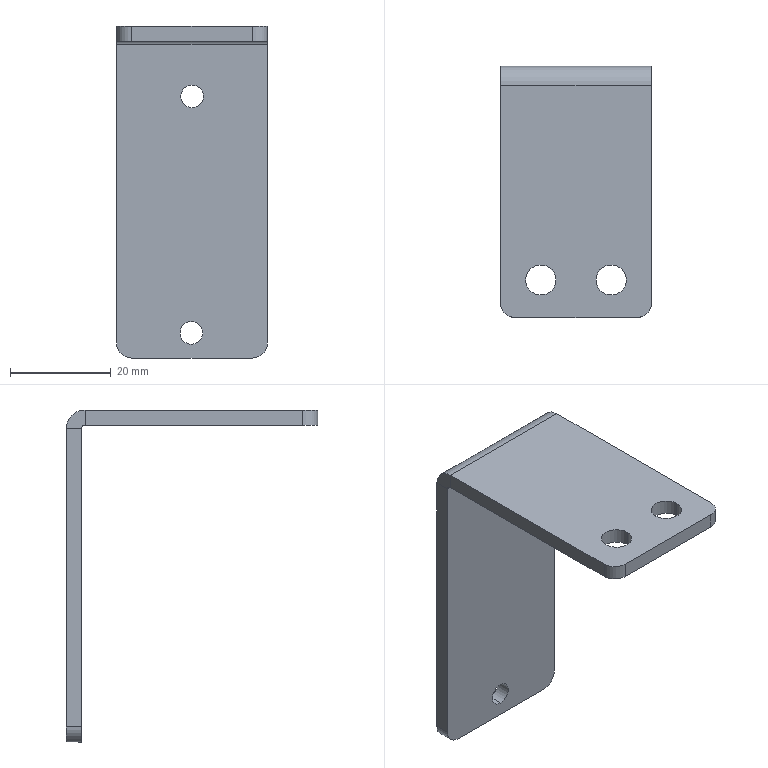Part | SolidWorks | features HoleWzd 2, EdgeFlange 1, Fillet 1, FlatPattern 1, SMBaseFlange 1, SheetMetal 1 | 1 solid | 26 faces | box 30 x 50 x 66 mm | volume 9795 mm3 | cylinder 14 | plane 12 | commonest cylinder face diameters 6 x8 4.5 x4 1.473 x1 7.473 x1
STEP:
#1=CARTESIAN_POINT('',(-0.1445,22.,-63.25));
#2=VERTEX_POINT('',#1);
#3=CARTESIAN_POINT('',(-0.1445,22.,-58.75));
#4=VERTEX_POINT('',#3);
#5=CARTESIAN_POINT('',(-0.1445,22.,-61.));
#6=DIRECTION('',(0.,1.,0.));
#7=DIRECTION('',(0.,0.,1.));
#8=AXIS2_PLACEMENT_3D('',#5,#6,#7);
#9=CIRCLE('',#8,2.25);
#10=EDGE_CURVE('',#2,#4,#9,.T.);
#11=ORIENTED_EDGE('',*,*,#10,.F.);
#12=CARTESIAN_POINT('',(-0.1445,25.,-63.25));
#13=VERTEX_POINT('',#12);
#14=CARTESIAN_POINT('',(-0.1445,25.,-63.25));
#15=DIRECTION('',(0.,1.,0.));
#16=VECTOR('',#15,1000.);
#17=LINE('',#14,#16);
#18=EDGE_CURVE('',#2,#13,#17,.T.);
#19=ORIENTED_EDGE('',*,*,#18,.T.);
#20=CARTESIAN_POINT('',(-0.1445,25.,-58.75));
#21=VERTEX_POINT('',#20);
#22=CARTESIAN_POINT('',(-0.1445,25.,-61.));
#23=DIRECTION('',(0.,1.,0.));
#24=DIRECTION('',(0.,0.,1.));
#25=AXIS2_PLACEMENT_3D('',#22,#23,#24);
#26=CIRCLE('',#25,2.25);
#27=EDGE_CURVE('',#13,#21,#26,.T.);
#28=ORIENTED_EDGE('',*,*,#27,.T.);
#29=CARTESIAN_POINT('',(-0.1445,25.,-58.75));
#30=DIRECTION('',(0.,1.,0.));
#31=VECTOR('',#30,1000.);
#32=LINE('',#29,#31);
#33=EDGE_CURVE('',#4,#21,#32,.T.);
#34=ORIENTED_EDGE('',*,*,#33,.F.);
#35=EDGE_LOOP('',(#11,#19,#28,#34));
#36=FACE_OUTER_BOUND('',#35,.T.);
#37=CARTESIAN_POINT('',(-0.1445,25.,-61.));
#38=DIRECTION('',(0.,1.,0.));
#39=DIRECTION('',(0.,0.,1.));
#40=AXIS2_PLACEMENT_3D('',#37,#38,#39);
#41=CYLINDRICAL_SURFACE('',#40,2.25);
#42=ADVANCED_FACE('',(#36),#41,.F.);
#43=CARTESIAN_POINT('',(0.0212,22.,-16.25));
#44=VERTEX_POINT('',#43);
#45=CARTESIAN_POINT('',(0.0212,22.,-11.75));
#46=VERTEX_POINT('',#45);
#47=CARTESIAN_POINT('',(0.0212,22.,-14.));
#48=DIRECTION('',(0.,1.,0.));
#49=DIRECTION('',(0.,0.,1.));
#50=AXIS2_PLACEMENT_3D('',#47,#48,#49);
#51=CIRCLE('',#50,2.25);
#52=EDGE_CURVE('',#44,#46,#51,.T.);
#53=ORIENTED_EDGE('',*,*,#52,.F.);
#54=CARTESIAN_POINT('',(0.0212,25.,-16.25));
#55=VERTEX_POINT('',#54);
#56=CARTESIAN_POINT('',(0.0212,25.,-16.25));
#57=DIRECTION('',(0.,1.,0.));
#58=VECTOR('',#57,1000.);
#59=LINE('',#56,#58);
#60=EDGE_CURVE('',#44,#55,#59,.T.);
#61=ORIENTED_EDGE('',*,*,#60,.T.);
#62=CARTESIAN_POINT('',(0.0212,25.,-11.75));
#63=VERTEX_POINT('',#62);
#64=CARTESIAN_POINT('',(0.0212,25.,-14.));
#65=DIRECTION('',(0.,1.,0.));
#66=DIRECTION('',(0.,0.,1.));
#67=AXIS2_PLACEMENT_3D('',#64,#65,#66);
#68=CIRCLE('',#67,2.25);
#69=EDGE_CURVE('',#55,#63,#68,.T.);
#70=ORIENTED_EDGE('',*,*,#69,.T.);
#71=CARTESIAN_POINT('',(0.0212,25.,-11.75));
#72=DIRECTION('',(0.,1.,0.));
#73=VECTOR('',#72,1000.);
#74=LINE('',#71,#73);
#75=EDGE_CURVE('',#46,#63,#74,.T.);
#76=ORIENTED_EDGE('',*,*,#75,.F.);
#77=EDGE_LOOP('',(#53,#61,#70,#76));
#78=FACE_OUTER_BOUND('',#77,.T.);
#79=CARTESIAN_POINT('',(0.0212,25.,-14.));
#80=DIRECTION('',(0.,1.,0.));
#81=DIRECTION('',(0.,0.,1.));
#82=AXIS2_PLACEMENT_3D('',#79,#80,#81);
#83=CYLINDRICAL_SURFACE('',#82,2.25);
#84=ADVANCED_FACE('',(#78),#83,.F.);
#85=CARTESIAN_POINT('',(-10.,-17.5,-3.));
#86=VERTEX_POINT('',#85);
#87=CARTESIAN_POINT('',(-4.,-17.5,-3.));
#88=VERTEX_POINT('',#87);
#89=CARTESIAN_POINT('',(-7.,-17.5,-3.));
#90=DIRECTION('',(0.,0.,1.));
#91=DIRECTION('',(1.,0.,0.));
#92=AXIS2_PLACEMENT_3D('',#89,#90,#91);
#93=CIRCLE('',#92,3.);
#94=EDGE_CURVE('',#86,#88,#93,.T.);
#95=ORIENTED_EDGE('',*,*,#94,.F.);
#96=CARTESIAN_POINT('',(-10.,-17.5,0.));
#97=VERTEX_POINT('',#96);
#98=CARTESIAN_POINT('',(-10.,-17.5,0.));
#99=DIRECTION('',(0.,0.,1.));
#100=VECTOR('',#99,1000.);
#101=LINE('',#98,#100);
#102=EDGE_CURVE('',#86,#97,#101,.T.);
#103=ORIENTED_EDGE('',*,*,#102,.T.);
#104=CARTESIAN_POINT('',(-4.,-17.5,0.));
#105=VERTEX_POINT('',#104);
#106=CARTESIAN_POINT('',(-7.,-17.5,0.));
#107=DIRECTION('',(0.,0.,1.));
#108=DIRECTION('',(1.,0.,0.));
#109=AXIS2_PLACEMENT_3D('',#106,#107,#108);
#110=CIRCLE('',#109,3.);
#111=EDGE_CURVE('',#97,#105,#110,.T.);
#112=ORIENTED_EDGE('',*,*,#111,.T.);
#113=CARTESIAN_POINT('',(-4.,-17.5,0.));
#114=DIRECTION('',(0.,0.,1.));
#115=VECTOR('',#114,1000.);
#116=LINE('',#113,#115);
#117=EDGE_CURVE('',#88,#105,#116,.T.);
#118=ORIENTED_EDGE('',*,*,#117,.F.);
#119=EDGE_LOOP('',(#95,#103,#112,#118));
#120=FACE_OUTER_BOUND('',#119,.T.);
#121=CARTESIAN_POINT('',(-7.,-17.5,0.));
#122=DIRECTION('',(0.,0.,1.));
#123=DIRECTION('',(1.,0.,0.));
#124=AXIS2_PLACEMENT_3D('',#121,#122,#123);
#125=CYLINDRICAL_SURFACE('',#124,3.);
#126=ADVANCED_FACE('',(#120),#125,.F.);
#127=CARTESIAN_POINT('',(4.,-17.5,-3.));
#128=VERTEX_POINT('',#127);
#129=CARTESIAN_POINT('',(10.,-17.5,-3.));
#130=VERTEX_POINT('',#129);
#131=CARTESIAN_POINT('',(7.,-17.5,-3.));
#132=DIRECTION('',(0.,0.,1.));
#133=DIRECTION('',(1.,0.,0.));
#134=AXIS2_PLACEMENT_3D('',#131,#132,#133);
#135=CIRCLE('',#134,3.);
#136=EDGE_CURVE('',#128,#130,#135,.T.);
#137=ORIENTED_EDGE('',*,*,#136,.F.);
#138=CARTESIAN_POINT('',(4.,-17.5,0.));
#139=VERTEX_POINT('',#138);
#140=CARTESIAN_POINT('',(4.,-17.5,0.));
#141=DIRECTION('',(0.,0.,1.));
#142=VECTOR('',#141,1000.);
#143=LINE('',#140,#142);
#144=EDGE_CURVE('',#128,#139,#143,.T.);
#145=ORIENTED_EDGE('',*,*,#144,.T.);
#146=CARTESIAN_POINT('',(10.,-17.5,0.));
#147=VERTEX_POINT('',#146);
#148=CARTESIAN_POINT('',(7.,-17.5,0.));
#149=DIRECTION('',(0.,0.,1.));
#150=DIRECTION('',(1.,0.,0.));
#151=AXIS2_PLACEMENT_3D('',#148,#149,#150);
#152=CIRCLE('',#151,3.);
#153=EDGE_CURVE('',#139,#147,#152,.T.);
#154=ORIENTED_EDGE('',*,*,#153,.T.);
#155=CARTESIAN_POINT('',(10.,-17.5,0.));
#156=DIRECTION('',(0.,0.,1.));
#157=VECTOR('',#156,1000.);
#158=LINE('',#155,#157);
#159=EDGE_CURVE('',#130,#147,#158,.T.);
#160=ORIENTED_EDGE('',*,*,#159,.F.);
#161=EDGE_LOOP('',(#137,#145,#154,#160));
#162=FACE_OUTER_BOUND('',#161,.T.);
#163=CARTESIAN_POINT('',(7.,-17.5,0.));
#164=DIRECTION('',(0.,0.,1.));
#165=DIRECTION('',(1.,0.,0.));
#166=AXIS2_PLACEMENT_3D('',#163,#164,#165);
#167=CYLINDRICAL_SURFACE('',#166,3.);
#168=ADVANCED_FACE('',(#162),#167,.F.);
#169=CARTESIAN_POINT('',(15.,-22.,0.));
#170=VERTEX_POINT('',#169);
#171=CARTESIAN_POINT('',(15.,21.263,0.));
#172=VERTEX_POINT('',#171);
#173=CARTESIAN_POINT('',(15.,25.,0.));
#174=DIRECTION('',(0.,1.,0.));
#175=VECTOR('',#174,1000.);
#176=LINE('',#173,#175);
#177=EDGE_CURVE('',#170,#172,#176,.T.);
#178=ORIENTED_EDGE('',*,*,#177,.F.);
#179=CARTESIAN_POINT('',(15.,-22.,-3.));
#180=VERTEX_POINT('',#179);
#181=CARTESIAN_POINT('',(15.,-22.,-3.));
#182=DIRECTION('',(0.,0.,-1.));
#183=VECTOR('',#182,1000.);
#184=LINE('',#181,#183);
#185=EDGE_CURVE('',#170,#180,#184,.T.);
#186=ORIENTED_EDGE('',*,*,#185,.T.);
#187=CARTESIAN_POINT('',(15.,21.263,-3.));
#188=VERTEX_POINT('',#187);
#189=CARTESIAN_POINT('',(15.,25.,-3.));
#190=DIRECTION('',(0.,1.,0.));
#191=VECTOR('',#190,1000.);
#192=LINE('',#189,#191);
#193=EDGE_CURVE('',#180,#188,#192,.T.);
#194=ORIENTED_EDGE('',*,*,#193,.T.);
#195=CARTESIAN_POINT('',(15.,21.263,-3.));
#196=DIRECTION('',(0.,0.,1.));
#197=VECTOR('',#196,1000.);
#198=LINE('',#195,#197);
#199=EDGE_CURVE('',#188,#172,#198,.T.);
#200=ORIENTED_EDGE('',*,*,#199,.T.);
#201=EDGE_LOOP('',(#178,#186,#194,#200));
#202=FACE_OUTER_BOUND('',#201,.T.);
#203=CARTESIAN_POINT('',(15.,25.,-3.));
#204=DIRECTION('',(1.,0.,0.));
#205=DIRECTION('',(0.,1.,0.));
#206=AXIS2_PLACEMENT_3D('',#203,#204,#205);
#207=PLANE('',#206);
#208=ADVANCED_FACE('',(#202),#207,.T.);
#209=CARTESIAN_POINT('',(-7.,-17.5,-3.));
#210=DIRECTION('',(0.,0.,1.));
#211=DIRECTION('',(1.,0.,0.));
#212=AXIS2_PLACEMENT_3D('',#209,#210,#211);
#213=CIRCLE('',#212,3.);
#214=EDGE_CURVE('',#88,#86,#213,.T.);
#215=ORIENTED_EDGE('',*,*,#214,.T.);
#216=ORIENTED_EDGE('',*,*,#94,.T.);
#217=EDGE_LOOP('',(#215,#216));
#218=FACE_BOUND('',#217,.T.);
#219=CARTESIAN_POINT('',(7.,-17.5,-3.));
#220=DIRECTION('',(0.,0.,1.));
#221=DIRECTION('',(1.,0.,0.));
#222=AXIS2_PLACEMENT_3D('',#219,#220,#221);
#223=CIRCLE('',#222,3.);
#224=EDGE_CURVE('',#130,#128,#223,.T.);
#225=ORIENTED_EDGE('',*,*,#224,.T.);
#226=ORIENTED_EDGE('',*,*,#136,.T.);
#227=EDGE_LOOP('',(#225,#226));
#228=FACE_BOUND('',#227,.T.);
#229=CARTESIAN_POINT('',(-12.,-25.,-3.));
#230=VERTEX_POINT('',#229);
#231=CARTESIAN_POINT('',(12.,-25.,-3.));
#232=VERTEX_POINT('',#231);
#233=CARTESIAN_POINT('',(-15.,-25.,-3.));
#234=DIRECTION('',(1.,0.,0.));
#235=VECTOR('',#234,1000.);
#236=LINE('',#233,#235);
#237=EDGE_CURVE('',#230,#232,#236,.T.);
#238=ORIENTED_EDGE('',*,*,#237,.F.);
#239=CARTESIAN_POINT('',(-15.,-22.,-3.));
#240=VERTEX_POINT('',#239);
#241=CARTESIAN_POINT('',(-12.,-22.,-3.));
#242=DIRECTION('',(0.,0.,-1.));
#243=DIRECTION('',(1.,0.,0.));
#244=AXIS2_PLACEMENT_3D('',#241,#242,#243);
#245=CIRCLE('',#244,3.);
#246=EDGE_CURVE('',#230,#240,#245,.T.);
#247=ORIENTED_EDGE('',*,*,#246,.T.);
#248=CARTESIAN_POINT('',(-15.,21.263,-3.));
#249=VERTEX_POINT('',#248);
#250=CARTESIAN_POINT('',(-15.,25.,-3.));
#251=DIRECTION('',(0.,-1.,0.));
#252=VECTOR('',#251,1000.);
#253=LINE('',#250,#252);
#254=EDGE_CURVE('',#249,#240,#253,.T.);
#255=ORIENTED_EDGE('',*,*,#254,.F.);
#256=CARTESIAN_POINT('',(15.,21.263,-3.));
#257=DIRECTION('',(-1.,0.,0.));
#258=VECTOR('',#257,1000.);
#259=LINE('',#256,#258);
#260=EDGE_CURVE('',#188,#249,#259,.T.);
#261=ORIENTED_EDGE('',*,*,#260,.F.);
#262=ORIENTED_EDGE('',*,*,#193,.F.);
#263=CARTESIAN_POINT('',(12.,-22.,-3.));
#264=DIRECTION('',(0.,0.,-1.));
#265=DIRECTION('',(1.,0.,0.));
#266=AXIS2_PLACEMENT_3D('',#263,#264,#265);
#267=CIRCLE('',#266,3.);
#268=EDGE_CURVE('',#180,#232,#267,.T.);
#269=ORIENTED_EDGE('',*,*,#268,.T.);
#270=EDGE_LOOP('',(#238,#247,#255,#261,#262,#269));
#271=FACE_OUTER_BOUND('',#270,.T.);
#272=CARTESIAN_POINT('',(0.,0.,-3.));
#273=DIRECTION('',(0.,0.,1.));
#274=DIRECTION('',(1.,0.,0.));
#275=AXIS2_PLACEMENT_3D('',#272,#273,#274);
#276=PLANE('',#275);
#277=ADVANCED_FACE('',(#218,#228,#271),#276,.F.);
#278=CARTESIAN_POINT('',(-7.,-17.5,0.));
#279=DIRECTION('',(0.,0.,1.));
#280=DIRECTION('',(1.,0.,0.));
#281=AXIS2_PLACEMENT_3D('',#278,#279,#280);
#282=CIRCLE('',#281,3.);
#283=EDGE_CURVE('',#105,#97,#282,.T.);
#284=ORIENTED_EDGE('',*,*,#283,.F.);
#285=ORIENTED_EDGE('',*,*,#111,.F.);
#286=EDGE_LOOP('',(#284,#285));
#287=FACE_BOUND('',#286,.T.);
#288=CARTESIAN_POINT('',(7.,-17.5,0.));
#289=DIRECTION('',(0.,0.,1.));
#290=DIRECTION('',(1.,0.,0.));
#291=AXIS2_PLACEMENT_3D('',#288,#289,#290);
#292=CIRCLE('',#291,3.);
#293=EDGE_CURVE('',#147,#139,#292,.T.);
#294=ORIENTED_EDGE('',*,*,#293,.F.);
#295=ORIENTED_EDGE('',*,*,#153,.F.);
#296=EDGE_LOOP('',(#294,#295));
#297=FACE_BOUND('',#296,.T.);
#298=CARTESIAN_POINT('',(-15.,21.263,0.));
#299=VERTEX_POINT('',#298);
#300=CARTESIAN_POINT('',(-15.,-22.,0.));
#301=VERTEX_POINT('',#300);
#302=CARTESIAN_POINT('',(-15.,25.,0.));
#303=DIRECTION('',(0.,-1.,0.));
#304=VECTOR('',#303,1000.);
#305=LINE('',#302,#304);
#306=EDGE_CURVE('',#299,#301,#305,.T.);
#307=ORIENTED_EDGE('',*,*,#306,.T.);
#308=CARTESIAN_POINT('',(-12.,-25.,0.));
#309=VERTEX_POINT('',#308);
#310=CARTESIAN_POINT('',(-12.,-22.,0.));
#311=DIRECTION('',(0.,0.,1.));
#312=DIRECTION('',(1.,0.,0.));
#313=AXIS2_PLACEMENT_3D('',#310,#311,#312);
#314=CIRCLE('',#313,3.);
#315=EDGE_CURVE('',#301,#309,#314,.T.);
#316=ORIENTED_EDGE('',*,*,#315,.T.);
#317=CARTESIAN_POINT('',(12.,-25.,0.));
#318=VERTEX_POINT('',#317);
#319=CARTESIAN_POINT('',(-15.,-25.,0.));
#320=DIRECTION('',(1.,0.,0.));
#321=VECTOR('',#320,1000.);
#322=LINE('',#319,#321);
#323=EDGE_CURVE('',#309,#318,#322,.T.);
#324=ORIENTED_EDGE('',*,*,#323,.T.);
#325=CARTESIAN_POINT('',(12.,-22.,0.));
#326=DIRECTION('',(0.,0.,1.));
#327=DIRECTION('',(1.,0.,0.));
#328=AXIS2_PLACEMENT_3D('',#325,#326,#327);
#329=CIRCLE('',#328,3.);
#330=EDGE_CURVE('',#318,#170,#329,.T.);
#331=ORIENTED_EDGE('',*,*,#330,.T.);
#332=ORIENTED_EDGE('',*,*,#177,.T.);
#333=CARTESIAN_POINT('',(15.,21.263,0.));
#334=DIRECTION('',(-1.,0.,0.));
#335=VECTOR('',#334,1000.);
#336=LINE('',#333,#335);
#337=EDGE_CURVE('',#172,#299,#336,.T.);
#338=ORIENTED_EDGE('',*,*,#337,.T.);
#339=EDGE_LOOP('',(#307,#316,#324,#331,#332,#338));
#340=FACE_OUTER_BOUND('',#339,.T.);
#341=CARTESIAN_POINT('',(0.,0.,0.));
#342=DIRECTION('',(0.,0.,1.));
#343=DIRECTION('',(1.,0.,0.));
#344=AXIS2_PLACEMENT_3D('',#341,#342,#343);
#345=PLANE('',#344);
#346=ADVANCED_FACE('',(#287,#297,#340),#345,.T.);
#347=ORIENTED_EDGE('',*,*,#323,.F.);
#348=CARTESIAN_POINT('',(-12.,-25.,-3.));
#349=DIRECTION('',(0.,0.,-1.));
#350=VECTOR('',#349,1000.);
#351=LINE('',#348,#350);
#352=EDGE_CURVE('',#309,#230,#351,.T.);
#353=ORIENTED_EDGE('',*,*,#352,.T.);
#354=ORIENTED_EDGE('',*,*,#237,.T.);
#355=CARTESIAN_POINT('',(12.,-25.,-3.));
#356=DIRECTION('',(0.,0.,1.));
#357=VECTOR('',#356,1000.);
#358=LINE('',#355,#357);
#359=EDGE_CURVE('',#232,#318,#358,.T.);
#360=ORIENTED_EDGE('',*,*,#359,.T.);
#361=EDGE_LOOP('',(#347,#353,#354,#360));
#362=FACE_OUTER_BOUND('',#361,.T.);
#363=CARTESIAN_POINT('',(-15.,-25.,-3.));
#364=DIRECTION('',(0.,-1.,0.));
#365=DIRECTION('',(0.,0.,-1.));
#366=AXIS2_PLACEMENT_3D('',#363,#364,#365);
#367=PLANE('',#366);
#368=ADVANCED_FACE('',(#362),#367,.T.);
#369=ORIENTED_EDGE('',*,*,#254,.T.);
#370=CARTESIAN_POINT('',(-15.,-22.,-3.));
#371=DIRECTION('',(0.,0.,1.));
#372=VECTOR('',#371,1000.);
#373=LINE('',#370,#372);
#374=EDGE_CURVE('',#240,#301,#373,.T.);
#375=ORIENTED_EDGE('',*,*,#374,.T.);
#376=ORIENTED_EDGE('',*,*,#306,.F.);
#377=CARTESIAN_POINT('',(-15.,21.263,-3.));
#378=DIRECTION('',(0.,0.,1.));
#379=VECTOR('',#378,1000.);
#380=LINE('',#377,#379);
#381=EDGE_CURVE('',#249,#299,#380,.T.);
#382=ORIENTED_EDGE('',*,*,#381,.F.);
#383=EDGE_LOOP('',(#369,#375,#376,#382));
#384=FACE_OUTER_BOUND('',#383,.T.);
#385=CARTESIAN_POINT('',(-15.,25.,-3.));
#386=DIRECTION('',(-1.,0.,0.));
#387=DIRECTION('',(0.,-1.,0.));
#388=AXIS2_PLACEMENT_3D('',#385,#386,#387);
#389=PLANE('',#388);
#390=ADVANCED_FACE('',(#384),#389,.T.);
#391=CARTESIAN_POINT('',(-15.,22.,-3.737));
#392=VERTEX_POINT('',#391);
#393=CARTESIAN_POINT('',(-15.,25.,-3.737));
#394=VERTEX_POINT('',#393);
#395=CARTESIAN_POINT('',(-15.,25.,-3.737));
#396=DIRECTION('',(0.,1.,0.));
#397=VECTOR('',#396,1000.);
#398=LINE('',#395,#397);
#399=EDGE_CURVE('',#392,#394,#398,.T.);
#400=ORIENTED_EDGE('',*,*,#399,.F.);
#401=CARTESIAN_POINT('',(-15.,21.263,-3.737));
#402=DIRECTION('',(-1.,0.,0.));
#403=DIRECTION('',(0.,0.,-1.));
#404=AXIS2_PLACEMENT_3D('',#401,#402,#403);
#405=CIRCLE('',#404,0.7366);
#406=EDGE_CURVE('',#249,#392,#405,.T.);
#407=ORIENTED_EDGE('',*,*,#406,.F.);
#408=ORIENTED_EDGE('',*,*,#381,.T.);
#409=CARTESIAN_POINT('',(-15.,21.263,-3.737));
#410=DIRECTION('',(-1.,0.,0.));
#411=DIRECTION('',(0.,0.,-1.));
#412=AXIS2_PLACEMENT_3D('',#409,#410,#411);
#413=CIRCLE('',#412,3.737);
#414=EDGE_CURVE('',#299,#394,#413,.T.);
#415=ORIENTED_EDGE('',*,*,#414,.T.);
#416=EDGE_LOOP('',(#400,#407,#408,#415));
#417=FACE_OUTER_BOUND('',#416,.T.);
#418=CARTESIAN_POINT('',(-15.,21.263,-3.737));
#419=DIRECTION('',(-1.,0.,0.));
#420=DIRECTION('',(0.,0.,1.));
#421=AXIS2_PLACEMENT_3D('',#418,#419,#420);
#422=PLANE('',#421);
#423=ADVANCED_FACE('',(#417),#422,.T.);
#424=CARTESIAN_POINT('',(15.,22.,-3.737));
#425=VERTEX_POINT('',#424);
#426=CARTESIAN_POINT('',(15.,21.263,-3.737));
#427=DIRECTION('',(1.,0.,0.));
#428=DIRECTION('',(0.,0.,-1.));
#429=AXIS2_PLACEMENT_3D('',#426,#427,#428);
#430=CIRCLE('',#429,0.7366);
#431=EDGE_CURVE('',#425,#188,#430,.T.);
#432=ORIENTED_EDGE('',*,*,#431,.F.);
#433=CARTESIAN_POINT('',(15.,25.,-3.737));
#434=VERTEX_POINT('',#433);
#435=CARTESIAN_POINT('',(15.,22.,-3.737));
#436=DIRECTION('',(0.,1.,0.));
#437=VECTOR('',#436,1000.);
#438=LINE('',#435,#437);
#439=EDGE_CURVE('',#425,#434,#438,.T.);
#440=ORIENTED_EDGE('',*,*,#439,.T.);
#441=CARTESIAN_POINT('',(15.,21.263,-3.737));
#442=DIRECTION('',(1.,0.,0.));
#443=DIRECTION('',(0.,0.,-1.));
#444=AXIS2_PLACEMENT_3D('',#441,#442,#443);
#445=CIRCLE('',#444,3.737);
#446=EDGE_CURVE('',#434,#172,#445,.T.);
#447=ORIENTED_EDGE('',*,*,#446,.T.);
#448=ORIENTED_EDGE('',*,*,#199,.F.);
#449=EDGE_LOOP('',(#432,#440,#447,#448));
#450=FACE_OUTER_BOUND('',#449,.T.);
#451=CARTESIAN_POINT('',(15.,21.263,-3.737));
#452=DIRECTION('',(-1.,0.,0.));
#453=DIRECTION('',(0.,0.,1.));
#454=AXIS2_PLACEMENT_3D('',#451,#452,#453);
#455=PLANE('',#454);
#456=ADVANCED_FACE('',(#450),#455,.F.);
#457=ORIENTED_EDGE('',*,*,#337,.F.);
#458=ORIENTED_EDGE('',*,*,#446,.F.);
#459=CARTESIAN_POINT('',(0.,25.,-3.737));
#460=DIRECTION('',(1.,0.,0.));
#461=VECTOR('',#460,1000.);
#462=LINE('',#459,#461);
#463=EDGE_CURVE('',#394,#434,#462,.T.);
#464=ORIENTED_EDGE('',*,*,#463,.F.);
#465=ORIENTED_EDGE('',*,*,#414,.F.);
#466=EDGE_LOOP('',(#457,#458,#464,#465));
#467=FACE_OUTER_BOUND('',#466,.T.);
#468=CARTESIAN_POINT('',(15.,21.263,-3.737));
#469=DIRECTION('',(1.,0.,0.));
#470=DIRECTION('',(0.,1.,0.));
#471=AXIS2_PLACEMENT_3D('',#468,#469,#470);
#472=CYLINDRICAL_SURFACE('',#471,3.737);
#473=ADVANCED_FACE('',(#467),#472,.T.);
#474=ORIENTED_EDGE('',*,*,#260,.T.);
#475=ORIENTED_EDGE('',*,*,#406,.T.);
#476=CARTESIAN_POINT('',(-15.,22.,-3.737));
#477=DIRECTION('',(1.,0.,0.));
#478=VECTOR('',#477,1000.);
#479=LINE('',#476,#478);
#480=EDGE_CURVE('',#392,#425,#479,.T.);
#481=ORIENTED_EDGE('',*,*,#480,.T.);
#482=ORIENTED_EDGE('',*,*,#431,.T.);
#483=EDGE_LOOP('',(#474,#475,#481,#482));
#484=FACE_OUTER_BOUND('',#483,.T.);
#485=CARTESIAN_POINT('',(15.,21.263,-3.737));
#486=DIRECTION('',(1.,0.,0.));
#487=DIRECTION('',(0.,1.,0.));
#488=AXIS2_PLACEMENT_3D('',#485,#486,#487);
#489=CYLINDRICAL_SURFACE('',#488,0.7366);
#490=ADVANCED_FACE('',(#484),#489,.F.);
#491=CARTESIAN_POINT('',(15.,22.,-63.));
#492=VERTEX_POINT('',#491);
#493=CARTESIAN_POINT('',(15.,22.,0.));
#494=DIRECTION('',(0.,0.,1.));
#495=VECTOR('',#494,1000.);
#496=LINE('',#493,#495);
#497=EDGE_CURVE('',#492,#425,#496,.T.);
#498=ORIENTED_EDGE('',*,*,#497,.F.);
#499=CARTESIAN_POINT('',(15.,25.,-63.));
#500=VERTEX_POINT('',#499);
#501=CARTESIAN_POINT('',(15.,25.,-63.));
#502=DIRECTION('',(0.,1.,0.));
#503=VECTOR('',#502,1000.);
#504=LINE('',#501,#503);
#505=EDGE_CURVE('',#492,#500,#504,.T.);
#506=ORIENTED_EDGE('',*,*,#505,.T.);
#507=CARTESIAN_POINT('',(15.,25.,-3.));
#508=DIRECTION('',(0.,0.,1.));
#509=VECTOR('',#508,1000.);
#510=LINE('',#507,#509);
#511=EDGE_CURVE('',#500,#434,#510,.T.);
#512=ORIENTED_EDGE('',*,*,#511,.T.);
#513=ORIENTED_EDGE('',*,*,#439,.F.);
#514=EDGE_LOOP('',(#498,#506,#512,#513));
#515=FACE_OUTER_BOUND('',#514,.T.);
#516=CARTESIAN_POINT('',(15.,25.,-3.));
#517=DIRECTION('',(1.,0.,0.));
#518=DIRECTION('',(0.,0.,-1.));
#519=AXIS2_PLACEMENT_3D('',#516,#517,#518);
#520=PLANE('',#519);
#521=ADVANCED_FACE('',(#515),#520,.T.);
#522=CARTESIAN_POINT('',(-15.,25.,-63.));
#523=VERTEX_POINT('',#522);
#524=CARTESIAN_POINT('',(-15.,25.,-66.));
#525=DIRECTION('',(0.,0.,-1.));
#526=VECTOR('',#525,1000.);
#527=LINE('',#524,#526);
#528=EDGE_CURVE('',#394,#523,#527,.T.);
#529=ORIENTED_EDGE('',*,*,#528,.T.);
#530=CARTESIAN_POINT('',(-15.,22.,-63.));
#531=VERTEX_POINT('',#530);
#532=CARTESIAN_POINT('',(-15.,25.,-63.));
#533=DIRECTION('',(0.,-1.,0.));
#534=VECTOR('',#533,1000.);
#535=LINE('',#532,#534);
#536=EDGE_CURVE('',#523,#531,#535,.T.);
#537=ORIENTED_EDGE('',*,*,#536,.T.);
#538=CARTESIAN_POINT('',(-15.,22.,0.));
#539=DIRECTION('',(0.,0.,-1.));
#540=VECTOR('',#539,1000.);
#541=LINE('',#538,#540);
#542=EDGE_CURVE('',#392,#531,#541,.T.);
#543=ORIENTED_EDGE('',*,*,#542,.F.);
#544=ORIENTED_EDGE('',*,*,#399,.T.);
#545=EDGE_LOOP('',(#529,#537,#543,#544));
#546=FACE_OUTER_BOUND('',#545,.T.);
#547=CARTESIAN_POINT('',(-15.,25.,-66.));
#548=DIRECTION('',(-1.,0.,0.));
#549=DIRECTION('',(0.,0.,1.));
#550=AXIS2_PLACEMENT_3D('',#547,#548,#549);
#551=PLANE('',#550);
#552=ADVANCED_FACE('',(#546),#551,.T.);
#553=CARTESIAN_POINT('',(-0.1445,25.,-61.));
#554=DIRECTION('',(0.,1.,0.));
#555=DIRECTION('',(0.,0.,1.));
#556=AXIS2_PLACEMENT_3D('',#553,#554,#555);
#557=CIRCLE('',#556,2.25);
#558=EDGE_CURVE('',#21,#13,#557,.T.);
#559=ORIENTED_EDGE('',*,*,#558,.F.);
#560=ORIENTED_EDGE('',*,*,#27,.F.);
#561=EDGE_LOOP('',(#559,#560));
#562=FACE_BOUND('',#561,.T.);
#563=CARTESIAN_POINT('',(0.0212,25.,-14.));
#564=DIRECTION('',(0.,1.,0.));
#565=DIRECTION('',(0.,0.,1.));
#566=AXIS2_PLACEMENT_3D('',#563,#564,#565);
#567=CIRCLE('',#566,2.25);
#568=EDGE_CURVE('',#63,#55,#567,.T.);
#569=ORIENTED_EDGE('',*,*,#568,.F.);
#570=ORIENTED_EDGE('',*,*,#69,.F.);
#571=EDGE_LOOP('',(#569,#570));
#572=FACE_BOUND('',#571,.T.);
#573=CARTESIAN_POINT('',(-12.,25.,-66.));
#574=VERTEX_POINT('',#573);
#575=CARTESIAN_POINT('',(12.,25.,-66.));
#576=VERTEX_POINT('',#575);
#577=CARTESIAN_POINT('',(15.,25.,-66.));
#578=DIRECTION('',(1.,0.,0.));
#579=VECTOR('',#578,1000.);
#580=LINE('',#577,#579);
#581=EDGE_CURVE('',#574,#576,#580,.T.);
#582=ORIENTED_EDGE('',*,*,#581,.F.);
#583=CARTESIAN_POINT('',(-12.,25.,-63.));
#584=DIRECTION('',(0.,1.,0.));
#585=DIRECTION('',(0.,0.,1.));
#586=AXIS2_PLACEMENT_3D('',#583,#584,#585);
#587=CIRCLE('',#586,3.);
#588=EDGE_CURVE('',#574,#523,#587,.T.);
#589=ORIENTED_EDGE('',*,*,#588,.T.);
#590=ORIENTED_EDGE('',*,*,#528,.F.);
#591=ORIENTED_EDGE('',*,*,#463,.T.);
#592=ORIENTED_EDGE('',*,*,#511,.F.);
#593=CARTESIAN_POINT('',(12.,25.,-63.));
#594=DIRECTION('',(0.,1.,0.));
#595=DIRECTION('',(0.,0.,1.));
#596=AXIS2_PLACEMENT_3D('',#593,#594,#595);
#597=CIRCLE('',#596,3.);
#598=EDGE_CURVE('',#500,#576,#597,.T.);
#599=ORIENTED_EDGE('',*,*,#598,.T.);
#600=EDGE_LOOP('',(#582,#589,#590,#591,#592,#599));
#601=FACE_OUTER_BOUND('',#600,.T.);
#602=CARTESIAN_POINT('',(0.,25.,0.));
#603=DIRECTION('',(0.,1.,0.));
#604=DIRECTION('',(0.,0.,1.));
#605=AXIS2_PLACEMENT_3D('',#602,#603,#604);
#606=PLANE('',#605);
#607=ADVANCED_FACE('',(#562,#572,#601),#606,.T.);
#608=CARTESIAN_POINT('',(-0.1445,22.,-61.));
#609=DIRECTION('',(0.,1.,0.));
#610=DIRECTION('',(0.,0.,1.));
#611=AXIS2_PLACEMENT_3D('',#608,#609,#610);
#612=CIRCLE('',#611,2.25);
#613=EDGE_CURVE('',#4,#2,#612,.T.);
#614=ORIENTED_EDGE('',*,*,#613,.T.);
#615=ORIENTED_EDGE('',*,*,#10,.T.);
#616=EDGE_LOOP('',(#614,#615));
#617=FACE_BOUND('',#616,.T.);
#618=CARTESIAN_POINT('',(0.0212,22.,-14.));
#619=DIRECTION('',(0.,1.,0.));
#620=DIRECTION('',(0.,0.,1.));
#621=AXIS2_PLACEMENT_3D('',#618,#619,#620);
#622=CIRCLE('',#621,2.25);
#623=EDGE_CURVE('',#46,#44,#622,.T.);
#624=ORIENTED_EDGE('',*,*,#623,.T.);
#625=ORIENTED_EDGE('',*,*,#52,.T.);
#626=EDGE_LOOP('',(#624,#625));
#627=FACE_BOUND('',#626,.T.);
#628=ORIENTED_EDGE('',*,*,#542,.T.);
#629=CARTESIAN_POINT('',(-12.,22.,-66.));
#630=VERTEX_POINT('',#629);
#631=CARTESIAN_POINT('',(-12.,22.,-63.));
#632=DIRECTION('',(0.,-1.,0.));
#633=DIRECTION('',(0.,0.,1.));
#634=AXIS2_PLACEMENT_3D('',#631,#632,#633);
#635=CIRCLE('',#634,3.);
#636=EDGE_CURVE('',#531,#630,#635,.T.);
#637=ORIENTED_EDGE('',*,*,#636,.T.);
#638=CARTESIAN_POINT('',(12.,22.,-66.));
#639=VERTEX_POINT('',#638);
#640=CARTESIAN_POINT('',(0.,22.,-66.));
#641=DIRECTION('',(1.,0.,0.));
#642=VECTOR('',#641,1000.);
#643=LINE('',#640,#642);
#644=EDGE_CURVE('',#630,#639,#643,.T.);
#645=ORIENTED_EDGE('',*,*,#644,.T.);
#646=CARTESIAN_POINT('',(12.,22.,-63.));
#647=DIRECTION('',(0.,-1.,0.));
#648=DIRECTION('',(0.,0.,1.));
#649=AXIS2_PLACEMENT_3D('',#646,#647,#648);
#650=CIRCLE('',#649,3.);
#651=EDGE_CURVE('',#639,#492,#650,.T.);
#652=ORIENTED_EDGE('',*,*,#651,.T.);
#653=ORIENTED_EDGE('',*,*,#497,.T.);
#654=ORIENTED_EDGE('',*,*,#480,.F.);
#655=EDGE_LOOP('',(#628,#637,#645,#652,#653,#654));
#656=FACE_OUTER_BOUND('',#655,.T.);
#657=CARTESIAN_POINT('',(0.,22.,0.));
#658=DIRECTION('',(0.,1.,0.));
#659=DIRECTION('',(0.,0.,1.));
#660=AXIS2_PLACEMENT_3D('',#657,#658,#659);
#661=PLANE('',#660);
#662=ADVANCED_FACE('',(#617,#627,#656),#661,.F.);
#663=ORIENTED_EDGE('',*,*,#644,.F.);
#664=CARTESIAN_POINT('',(-12.,25.,-66.));
#665=DIRECTION('',(0.,1.,0.));
#666=VECTOR('',#665,1000.);
#667=LINE('',#664,#666);
#668=EDGE_CURVE('',#630,#574,#667,.T.);
#669=ORIENTED_EDGE('',*,*,#668,.T.);
#670=ORIENTED_EDGE('',*,*,#581,.T.);
#671=CARTESIAN_POINT('',(12.,25.,-66.));
#672=DIRECTION('',(0.,-1.,0.));
#673=VECTOR('',#672,1000.);
#674=LINE('',#671,#673);
#675=EDGE_CURVE('',#576,#639,#674,.T.);
#676=ORIENTED_EDGE('',*,*,#675,.T.);
#677=EDGE_LOOP('',(#663,#669,#670,#676));
#678=FACE_OUTER_BOUND('',#677,.T.);
#679=CARTESIAN_POINT('',(15.,25.,-66.));
#680=DIRECTION('',(0.,0.,-1.));
#681=DIRECTION('',(0.,1.,0.));
#682=AXIS2_PLACEMENT_3D('',#679,#680,#681);
#683=PLANE('',#682);
#684=ADVANCED_FACE('',(#678),#683,.T.);
#685=ORIENTED_EDGE('',*,*,#144,.F.);
#686=ORIENTED_EDGE('',*,*,#224,.F.);
#687=ORIENTED_EDGE('',*,*,#159,.T.);
#688=ORIENTED_EDGE('',*,*,#293,.T.);
#689=EDGE_LOOP('',(#685,#686,#687,#688));
#690=FACE_OUTER_BOUND('',#689,.T.);
#691=CARTESIAN_POINT('',(7.,-17.5,0.));
#692=DIRECTION('',(0.,0.,1.));
#693=DIRECTION('',(1.,0.,0.));
#694=AXIS2_PLACEMENT_3D('',#691,#692,#693);
#695=CYLINDRICAL_SURFACE('',#694,3.);
#696=ADVANCED_FACE('',(#690),#695,.F.);
#697=ORIENTED_EDGE('',*,*,#102,.F.);
#698=ORIENTED_EDGE('',*,*,#214,.F.);
#699=ORIENTED_EDGE('',*,*,#117,.T.);
#700=ORIENTED_EDGE('',*,*,#283,.T.);
#701=EDGE_LOOP('',(#697,#698,#699,#700));
#702=FACE_OUTER_BOUND('',#701,.T.);
#703=CARTESIAN_POINT('',(-7.,-17.5,0.));
#704=DIRECTION('',(0.,0.,1.));
#705=DIRECTION('',(1.,0.,0.));
#706=AXIS2_PLACEMENT_3D('',#703,#704,#705);
#707=CYLINDRICAL_SURFACE('',#706,3.);
#708=ADVANCED_FACE('',(#702),#707,.F.);
#709=ORIENTED_EDGE('',*,*,#246,.F.);
#710=ORIENTED_EDGE('',*,*,#352,.F.);
#711=ORIENTED_EDGE('',*,*,#315,.F.);
#712=ORIENTED_EDGE('',*,*,#374,.F.);
#713=EDGE_LOOP('',(#709,#710,#711,#712));
#714=FACE_OUTER_BOUND('',#713,.T.);
#715=CARTESIAN_POINT('',(-12.,-22.,-3.));
#716=DIRECTION('',(0.,0.,1.));
#717=DIRECTION('',(1.,0.,0.));
#718=AXIS2_PLACEMENT_3D('',#715,#716,#717);
#719=CYLINDRICAL_SURFACE('',#718,3.);
#720=ADVANCED_FACE('',(#714),#719,.T.);
#721=ORIENTED_EDGE('',*,*,#268,.F.);
#722=ORIENTED_EDGE('',*,*,#185,.F.);
#723=ORIENTED_EDGE('',*,*,#330,.F.);
#724=ORIENTED_EDGE('',*,*,#359,.F.);
#725=EDGE_LOOP('',(#721,#722,#723,#724));
#726=FACE_OUTER_BOUND('',#725,.T.);
#727=CARTESIAN_POINT('',(12.,-22.,-3.));
#728=DIRECTION('',(0.,0.,1.));
#729=DIRECTION('',(1.,0.,0.));
#730=AXIS2_PLACEMENT_3D('',#727,#728,#729);
#731=CYLINDRICAL_SURFACE('',#730,3.);
#732=ADVANCED_FACE('',(#726),#731,.T.);
#733=ORIENTED_EDGE('',*,*,#588,.F.);
#734=ORIENTED_EDGE('',*,*,#668,.F.);
#735=ORIENTED_EDGE('',*,*,#636,.F.);
#736=ORIENTED_EDGE('',*,*,#536,.F.);
#737=EDGE_LOOP('',(#733,#734,#735,#736));
#738=FACE_OUTER_BOUND('',#737,.T.);
#739=CARTESIAN_POINT('',(-12.,25.,-63.));
#740=DIRECTION('',(0.,-1.,0.));
#741=DIRECTION('',(0.,0.,-1.));
#742=AXIS2_PLACEMENT_3D('',#739,#740,#741);
#743=CYLINDRICAL_SURFACE('',#742,3.);
#744=ADVANCED_FACE('',(#738),#743,.T.);
#745=ORIENTED_EDGE('',*,*,#598,.F.);
#746=ORIENTED_EDGE('',*,*,#505,.F.);
#747=ORIENTED_EDGE('',*,*,#651,.F.);
#748=ORIENTED_EDGE('',*,*,#675,.F.);
#749=EDGE_LOOP('',(#745,#746,#747,#748));
#750=FACE_OUTER_BOUND('',#749,.T.);
#751=CARTESIAN_POINT('',(12.,25.,-63.));
#752=DIRECTION('',(0.,-1.,0.));
#753=DIRECTION('',(0.,0.,-1.));
#754=AXIS2_PLACEMENT_3D('',#751,#752,#753);
#755=CYLINDRICAL_SURFACE('',#754,3.);
#756=ADVANCED_FACE('',(#750),#755,.T.);
#757=ORIENTED_EDGE('',*,*,#60,.F.);
#758=ORIENTED_EDGE('',*,*,#623,.F.);
#759=ORIENTED_EDGE('',*,*,#75,.T.);
#760=ORIENTED_EDGE('',*,*,#568,.T.);
#761=EDGE_LOOP('',(#757,#758,#759,#760));
#762=FACE_OUTER_BOUND('',#761,.T.);
#763=CARTESIAN_POINT('',(0.0212,25.,-14.));
#764=DIRECTION('',(0.,1.,0.));
#765=DIRECTION('',(0.,0.,1.));
#766=AXIS2_PLACEMENT_3D('',#763,#764,#765);
#767=CYLINDRICAL_SURFACE('',#766,2.25);
#768=ADVANCED_FACE('',(#762),#767,.F.);
#769=ORIENTED_EDGE('',*,*,#18,.F.);
#770=ORIENTED_EDGE('',*,*,#613,.F.);
#771=ORIENTED_EDGE('',*,*,#33,.T.);
#772=ORIENTED_EDGE('',*,*,#558,.T.);
#773=EDGE_LOOP('',(#769,#770,#771,#772));
#774=FACE_OUTER_BOUND('',#773,.T.);
#775=CARTESIAN_POINT('',(-0.1445,25.,-61.));
#776=DIRECTION('',(0.,1.,0.));
#777=DIRECTION('',(0.,0.,1.));
#778=AXIS2_PLACEMENT_3D('',#775,#776,#777);
#779=CYLINDRICAL_SURFACE('',#778,2.25);
#780=ADVANCED_FACE('',(#774),#779,.F.);
#781=CLOSED_SHELL('',(#42,#84,#126,#168,#208,#277,#346,#368,#390,#423,#456,#473,#490,#521,#552,#607,#662,#684,#696,#708,#720,#732,#744,#756,#768,#780));
#782=MANIFOLD_SOLID_BREP('',#781);
#783=CARTESIAN_POINT('',(0.,0.,0.));
#784=DIRECTION('',(0.,0.,1.));
#785=DIRECTION('',(1.,0.,0.));
#786=AXIS2_PLACEMENT_3D('',#783,#784,#785);
#787=(LENGTH_UNIT()NAMED_UNIT(*)SI_UNIT(.MILLI.,.METRE.));
#788=UNCERTAINTY_MEASURE_WITH_UNIT(LENGTH_MEASURE(0.00001),#787,'','');
#789=(NAMED_UNIT(*)PLANE_ANGLE_UNIT()SI_UNIT($,.RADIAN.));
#790=(NAMED_UNIT(*)SI_UNIT($,.STERADIAN.)SOLID_ANGLE_UNIT());
#791=(GEOMETRIC_REPRESENTATION_CONTEXT(3)GLOBAL_UNCERTAINTY_ASSIGNED_CONTEXT((#788))GLOBAL_UNIT_ASSIGNED_CONTEXT((#787,#789,#790))REPRESENTATION_CONTEXT('',''));
#792=ADVANCED_BREP_SHAPE_REPRESENTATION('',(#782,#786),#791);